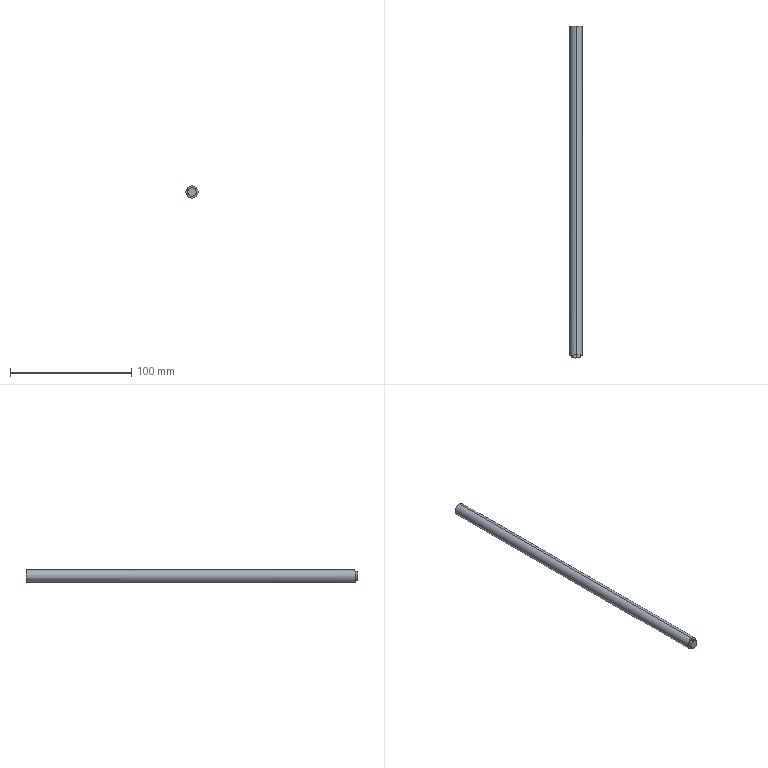Part | Creo | 1 solid | 8 faces | box 10 x 273.752 x 10 mm | volume 21397 mm3 | plane 4 | cylinder 4 | commonest cylinder face diameters 7.035 x2 10 x2
STEP:
#1=CARTESIAN_POINT('',(0.,0.,0.));
#2=DIRECTION('',(0.,0.,1.));
#3=DIRECTION('',(1.,0.,0.));
#4=AXIS2_PLACEMENT_3D('',#1,#2,#3);
#5=CARTESIAN_POINT('',(90.074,305.373,-76.269));
#6=VERTEX_POINT('',#5);
#7=CARTESIAN_POINT('',(85.074,305.373,-81.269));
#8=VERTEX_POINT('',#7);
#9=CARTESIAN_POINT('',(85.074,305.373,-76.269));
#10=DIRECTION('',(0.,1.,0.));
#11=DIRECTION('',(1.,0.,0.));
#12=AXIS2_PLACEMENT_3D('',#9,#10,#11);
#13=CIRCLE('',#12,5.);
#14=EDGE_CURVE('',#6,#8,#13,.T.);
#15=ORIENTED_EDGE('',*,*,#14,.F.);
#16=CARTESIAN_POINT('',(85.074,305.373,-71.269));
#17=VERTEX_POINT('',#16);
#18=CARTESIAN_POINT('',(85.074,305.373,-76.269));
#19=DIRECTION('',(0.,1.,0.));
#20=DIRECTION('',(0.,0.,1.));
#21=AXIS2_PLACEMENT_3D('',#18,#19,#20);
#22=CIRCLE('',#21,5.);
#23=EDGE_CURVE('',#17,#6,#22,.T.);
#24=ORIENTED_EDGE('',*,*,#23,.F.);
#25=CARTESIAN_POINT('',(85.074,305.373,-76.269));
#26=DIRECTION('',(0.,1.,0.));
#27=DIRECTION('',(0.,0.,-1.));
#28=AXIS2_PLACEMENT_3D('',#25,#26,#27);
#29=CIRCLE('',#28,5.);
#30=EDGE_CURVE('',#8,#17,#29,.T.);
#31=ORIENTED_EDGE('',*,*,#30,.F.);
#32=EDGE_LOOP('',(#15,#24,#31));
#33=FACE_OUTER_BOUND('',#32,.F.);
#34=CARTESIAN_POINT('',(-335.899,305.373,-228.441));
#35=DIRECTION('',(0.,-1.,0.));
#36=DIRECTION('',(1.,0.,0.));
#37=AXIS2_PLACEMENT_3D('',#34,#35,#36);
#38=PLANE('',#37);
#39=ADVANCED_FACE('',(#33),#38,.F.);
#40=CARTESIAN_POINT('',(85.074,34.139,-71.269));
#41=VERTEX_POINT('',#40);
#42=CARTESIAN_POINT('',(85.075,33.964,-81.269));
#43=VERTEX_POINT('',#42);
#44=CARTESIAN_POINT('',(85.074,34.139,-71.269));
#45=CARTESIAN_POINT('',(85.307,34.139,-71.269));
#46=CARTESIAN_POINT('',(85.767,34.139,-71.301));
#47=CARTESIAN_POINT('',(86.449,34.137,-71.445));
#48=CARTESIAN_POINT('',(87.103,34.133,-71.682));
#49=CARTESIAN_POINT('',(87.718,34.128,-72.007));
#50=CARTESIAN_POINT('',(88.283,34.121,-72.414));
#51=CARTESIAN_POINT('',(88.785,34.113,-72.895));
#52=CARTESIAN_POINT('',(89.217,34.104,-73.441));
#53=CARTESIAN_POINT('',(89.568,34.094,-74.042));
#54=CARTESIAN_POINT('',(89.833,34.083,-74.685));
#55=CARTESIAN_POINT('',(90.007,34.071,-75.359));
#56=CARTESIAN_POINT('',(90.085,34.059,-76.051));
#57=CARTESIAN_POINT('',(90.067,34.047,-76.746));
#58=CARTESIAN_POINT('',(89.953,34.035,-77.433));
#59=CARTESIAN_POINT('',(89.745,34.023,-78.097));
#60=CARTESIAN_POINT('',(89.447,34.012,-78.726));
#61=CARTESIAN_POINT('',(89.065,34.002,-79.307));
#62=CARTESIAN_POINT('',(88.606,33.992,-79.831));
#63=CARTESIAN_POINT('',(88.079,33.984,-80.285));
#64=CARTESIAN_POINT('',(87.494,33.977,-80.662));
#65=CARTESIAN_POINT('',(86.86,33.971,-80.956));
#66=CARTESIAN_POINT('',(86.218,33.967,-81.149));
#67=CARTESIAN_POINT('',(85.657,33.965,-81.246));
#68=CARTESIAN_POINT('',(85.266,33.964,-81.269));
#69=CARTESIAN_POINT('',(85.075,33.964,-81.269));
#70=B_SPLINE_CURVE_WITH_KNOTS('',3,(#44,#45,#46,#47,#48,#49,#50,#51,#52,#53,#54,#55,#56,#57,#58,#59,#60,#61,#62,#63,#64,#65,#66,#67,#68,#69),.UNSPECIFIED.,.F.,.F.,(4,1,1,1,1,1,1,1,1,1,1,1,1,1,1,1,1,1,1,1,1,1,1,4),(0.,0.04348,0.08696,0.1304,0.1739,0.2174,0.2609,0.3043,0.3478,0.3913,0.4348,0.4783,0.5217,0.5652,0.6087,0.6522,0.6957,0.7391,0.7826,0.8261,0.8696,0.913,0.9565,1.),.UNSPECIFIED.);
#71=EDGE_CURVE('',#41,#43,#70,.T.);
#72=ORIENTED_EDGE('',*,*,#71,.F.);
#73=CARTESIAN_POINT('',(85.074,34.139,-71.269));
#74=DIRECTION('',(0.,1.,0.000000528));
#75=VECTOR('',#74,271.234);
#76=LINE('',#73,#75);
#77=EDGE_CURVE('',#41,#17,#76,.T.);
#78=ORIENTED_EDGE('',*,*,#77,.T.);
#79=ORIENTED_EDGE('',*,*,#23,.T.);
#80=ORIENTED_EDGE('',*,*,#14,.T.);
#81=CARTESIAN_POINT('',(85.075,33.964,-81.269));
#82=DIRECTION('',(-0.000005033,1.,-0.00000083));
#83=VECTOR('',#82,271.408);
#84=LINE('',#81,#83);
#85=EDGE_CURVE('',#43,#8,#84,.T.);
#86=ORIENTED_EDGE('',*,*,#85,.F.);
#87=EDGE_LOOP('',(#72,#78,#79,#80,#86));
#88=FACE_OUTER_BOUND('',#87,.F.);
#89=CARTESIAN_POINT('',(85.074,34.051,-76.269));
#90=DIRECTION('',(0.,1.,0.));
#91=DIRECTION('',(0.,0.,1.));
#92=AXIS2_PLACEMENT_3D('',#89,#90,#91);
#93=CYLINDRICAL_SURFACE('',#92,5.);
#94=ADVANCED_FACE('',(#88),#93,.T.);
#95=ORIENTED_EDGE('',*,*,#71,.T.);
#96=CARTESIAN_POINT('',(84.837,33.964,-81.263));
#97=VERTEX_POINT('',#96);
#98=CARTESIAN_POINT('',(85.075,33.964,-81.269));
#99=CARTESIAN_POINT('',(84.995,33.964,-81.269));
#100=CARTESIAN_POINT('',(84.917,33.964,-81.267));
#101=CARTESIAN_POINT('',(84.837,33.964,-81.263));
#102=B_SPLINE_CURVE_WITH_KNOTS('',3,(#98,#99,#100,#101),.UNSPECIFIED.,.F.,.F.,(4,4),(0.,1.),.UNSPECIFIED.);
#103=EDGE_CURVE('',#43,#97,#102,.T.);
#104=ORIENTED_EDGE('',*,*,#103,.T.);
#105=CARTESIAN_POINT('',(81.074,33.996,-79.269));
#106=VERTEX_POINT('',#105);
#107=CARTESIAN_POINT('',(84.465,33.964,-81.246));
#108=CARTESIAN_POINT('',(83.745,33.965,-81.13));
#109=CARTESIAN_POINT('',(82.713,33.972,-80.723));
#110=CARTESIAN_POINT('',(81.797,33.982,-80.098));
#111=CARTESIAN_POINT('',(81.297,33.991,-79.567));
#112=CARTESIAN_POINT('',(81.074,33.996,-79.269));
#113=B_SPLINE_CURVE_WITH_KNOTS('',3,(#96,#107,#108,#109,#110,#111,#112),.UNSPECIFIED.,.F.,.F.,(4,1,1,1,4),(0.,0.25,0.5,0.75,1.),.UNSPECIFIED.);
#114=EDGE_CURVE('',#97,#106,#113,.T.);
#115=ORIENTED_EDGE('',*,*,#114,.T.);
#116=CARTESIAN_POINT('',(81.074,34.1,-73.269));
#117=VERTEX_POINT('',#116);
#118=CARTESIAN_POINT('',(81.074,34.1,-73.269));
#119=DIRECTION('',(-0.000000019,-0.01745,-0.9998));
#120=VECTOR('',#119,6.001);
#121=LINE('',#118,#120);
#122=EDGE_CURVE('',#117,#106,#121,.T.);
#123=ORIENTED_EDGE('',*,*,#122,.F.);
#124=CARTESIAN_POINT('',(81.074,34.1,-73.269));
#125=CARTESIAN_POINT('',(81.309,34.106,-72.955));
#126=CARTESIAN_POINT('',(81.839,34.116,-72.398));
#127=CARTESIAN_POINT('',(82.817,34.128,-71.756));
#128=CARTESIAN_POINT('',(83.918,34.136,-71.359));
#129=CARTESIAN_POINT('',(84.68,34.138,-71.269));
#130=CARTESIAN_POINT('',(85.074,34.139,-71.269));
#131=B_SPLINE_CURVE_WITH_KNOTS('',3,(#124,#125,#126,#127,#128,#129,#130),.UNSPECIFIED.,.F.,.F.,(4,1,1,1,4),(0.,0.25,0.5,0.75,1.),.UNSPECIFIED.);
#132=EDGE_CURVE('',#117,#41,#131,.T.);
#133=ORIENTED_EDGE('',*,*,#132,.T.);
#134=EDGE_LOOP('',(#95,#104,#115,#123,#133));
#135=FACE_OUTER_BOUND('',#134,.F.);
#136=CARTESIAN_POINT('',(85.074,34.113,-72.751));
#137=VERTEX_POINT('',#136);
#138=CARTESIAN_POINT('',(85.074,33.99,-79.786));
#139=VERTEX_POINT('',#138);
#140=CARTESIAN_POINT('',(85.074,34.113,-72.751));
#141=CARTESIAN_POINT('',(85.416,34.113,-72.751));
#142=CARTESIAN_POINT('',(86.072,34.112,-72.847));
#143=CARTESIAN_POINT('',(87.,34.105,-73.268));
#144=CARTESIAN_POINT('',(87.766,34.094,-73.933));
#145=CARTESIAN_POINT('',(88.314,34.08,-74.785));
#146=CARTESIAN_POINT('',(88.6,34.063,-75.752));
#147=CARTESIAN_POINT('',(88.604,34.046,-76.762));
#148=CARTESIAN_POINT('',(88.322,34.028,-77.738));
#149=CARTESIAN_POINT('',(87.775,34.013,-78.596));
#150=CARTESIAN_POINT('',(87.009,34.001,-79.264));
#151=CARTESIAN_POINT('',(86.083,33.993,-79.688));
#152=CARTESIAN_POINT('',(85.421,33.99,-79.786));
#153=CARTESIAN_POINT('',(85.074,33.99,-79.786));
#154=B_SPLINE_CURVE_WITH_KNOTS('',3,(#140,#141,#142,#143,#144,#145,#146,#147,#148,#149,#150,#151,#152,#153),.UNSPECIFIED.,.F.,.F.,(4,1,1,1,1,1,1,1,1,1,1,4),(0.,0.09091,0.1818,0.2727,0.3636,0.4545,0.5455,0.6364,0.7273,0.8182,0.9091,1.),.UNSPECIFIED.);
#155=EDGE_CURVE('',#137,#139,#154,.T.);
#156=ORIENTED_EDGE('',*,*,#155,.F.);
#157=CARTESIAN_POINT('',(84.907,33.99,-79.782));
#158=VERTEX_POINT('',#157);
#159=CARTESIAN_POINT('',(84.907,33.99,-79.782));
#160=CARTESIAN_POINT('',(84.53,33.99,-79.765));
#161=CARTESIAN_POINT('',(83.823,33.992,-79.615));
#162=CARTESIAN_POINT('',(82.858,34.001,-79.075));
#163=CARTESIAN_POINT('',(82.111,34.014,-78.268));
#164=CARTESIAN_POINT('',(81.642,34.031,-77.27));
#165=CARTESIAN_POINT('',(81.501,34.05,-76.172));
#166=CARTESIAN_POINT('',(81.699,34.069,-75.094));
#167=CARTESIAN_POINT('',(82.214,34.086,-74.125));
#168=CARTESIAN_POINT('',(83.003,34.101,-73.355));
#169=CARTESIAN_POINT('',(83.996,34.11,-72.863));
#170=CARTESIAN_POINT('',(84.702,34.112,-72.751));
#171=CARTESIAN_POINT('',(85.074,34.113,-72.751));
#172=B_SPLINE_CURVE_WITH_KNOTS('',3,(#159,#160,#161,#162,#163,#164,#165,#166,#167,#168,#169,#170,#171),.UNSPECIFIED.,.F.,.F.,(4,1,1,1,1,1,1,1,1,1,4),(0.,0.1,0.2,0.3,0.4,0.5,0.6,0.7,0.8,0.9,1.),.UNSPECIFIED.);
#173=EDGE_CURVE('',#158,#137,#172,.T.);
#174=ORIENTED_EDGE('',*,*,#173,.F.);
#175=CARTESIAN_POINT('',(85.074,33.99,-79.786));
#176=CARTESIAN_POINT('',(85.018,33.99,-79.786));
#177=CARTESIAN_POINT('',(84.962,33.99,-79.785));
#178=B_SPLINE_CURVE_WITH_KNOTS('',3,(#175,#176,#177,#157),.UNSPECIFIED.,.F.,.F.,(4,4),(0.,1.),.UNSPECIFIED.);
#179=EDGE_CURVE('',#139,#158,#178,.T.);
#180=ORIENTED_EDGE('',*,*,#179,.F.);
#181=EDGE_LOOP('',(#156,#174,#180));
#182=FACE_BOUND('',#181,.F.);
#183=CARTESIAN_POINT('',(82.032,34.202,-67.473));
#184=DIRECTION('',(-0.0008272,0.9998,-0.01745));
#185=DIRECTION('',(0.,0.01745,0.9998));
#186=AXIS2_PLACEMENT_3D('',#183,#184,#185);
#187=PLANE('',#186);
#188=ADVANCED_FACE('',(#135,#182),#187,.F.);
#189=CARTESIAN_POINT('',(81.074,33.996,-79.269));
#190=CARTESIAN_POINT('',(80.811,34.002,-78.918));
#191=CARTESIAN_POINT('',(80.393,34.014,-78.176));
#192=CARTESIAN_POINT('',(80.059,34.036,-76.917));
#193=CARTESIAN_POINT('',(80.059,34.059,-75.621));
#194=CARTESIAN_POINT('',(80.393,34.081,-74.362));
#195=CARTESIAN_POINT('',(80.811,34.094,-73.62));
#196=CARTESIAN_POINT('',(81.074,34.1,-73.269));
#197=B_SPLINE_CURVE_WITH_KNOTS('',3,(#189,#190,#191,#192,#193,#194,#195,#196),.UNSPECIFIED.,.F.,.F.,(4,1,1,1,1,4),(0.,0.2,0.4,0.6,0.8,1.),.UNSPECIFIED.);
#198=EDGE_CURVE('',#106,#117,#197,.T.);
#199=ORIENTED_EDGE('',*,*,#198,.F.);
#200=ORIENTED_EDGE('',*,*,#114,.F.);
#201=ORIENTED_EDGE('',*,*,#103,.F.);
#202=ORIENTED_EDGE('',*,*,#85,.T.);
#203=ORIENTED_EDGE('',*,*,#30,.T.);
#204=ORIENTED_EDGE('',*,*,#77,.F.);
#205=ORIENTED_EDGE('',*,*,#132,.F.);
#206=EDGE_LOOP('',(#199,#200,#201,#202,#203,#204,#205));
#207=FACE_OUTER_BOUND('',#206,.F.);
#208=CARTESIAN_POINT('',(85.074,34.051,-76.269));
#209=DIRECTION('',(0.,1.,0.));
#210=DIRECTION('',(0.,0.,1.));
#211=AXIS2_PLACEMENT_3D('',#208,#209,#210);
#212=CYLINDRICAL_SURFACE('',#211,5.);
#213=ADVANCED_FACE('',(#207),#212,.T.);
#214=ORIENTED_EDGE('',*,*,#198,.T.);
#215=ORIENTED_EDGE('',*,*,#122,.T.);
#216=EDGE_LOOP('',(#214,#215));
#217=FACE_OUTER_BOUND('',#216,.F.);
#218=CARTESIAN_POINT('',(81.083,33.981,-80.128));
#219=DIRECTION('',(-0.0008272,0.9998,-0.01745));
#220=DIRECTION('',(0.,0.01745,0.9998));
#221=AXIS2_PLACEMENT_3D('',#218,#219,#220);
#222=PLANE('',#221);
#223=ADVANCED_FACE('',(#217),#222,.F.);
#224=ORIENTED_EDGE('',*,*,#155,.T.);
#225=CARTESIAN_POINT('',(85.074,31.744,-79.786));
#226=VERTEX_POINT('',#225);
#227=CARTESIAN_POINT('',(85.074,33.99,-79.786));
#228=DIRECTION('',(0.,-1.,0.));
#229=VECTOR('',#228,2.246);
#230=LINE('',#227,#229);
#231=EDGE_CURVE('',#139,#226,#230,.T.);
#232=ORIENTED_EDGE('',*,*,#231,.T.);
#233=CARTESIAN_POINT('',(85.074,31.621,-72.751));
#234=VERTEX_POINT('',#233);
#235=CARTESIAN_POINT('',(85.074,31.744,-79.786));
#236=CARTESIAN_POINT('',(85.488,31.744,-79.786));
#237=CARTESIAN_POINT('',(86.384,31.742,-79.635));
#238=CARTESIAN_POINT('',(87.635,31.729,-78.833));
#239=CARTESIAN_POINT('',(88.441,31.707,-77.57));
#240=CARTESIAN_POINT('',(88.666,31.685,-76.269));
#241=CARTESIAN_POINT('',(88.441,31.662,-74.968));
#242=CARTESIAN_POINT('',(87.635,31.639,-73.705));
#243=CARTESIAN_POINT('',(86.384,31.624,-72.902));
#244=CARTESIAN_POINT('',(85.488,31.621,-72.751));
#245=CARTESIAN_POINT('',(85.074,31.621,-72.751));
#246=B_SPLINE_CURVE_WITH_KNOTS('',3,(#235,#236,#237,#238,#239,#240,#241,#242,#243,#244,#245),.UNSPECIFIED.,.F.,.F.,(4,1,1,1,1,1,1,1,4),(0.,0.125,0.25,0.375,0.5,0.625,0.75,0.875,1.),.UNSPECIFIED.);
#247=EDGE_CURVE('',#226,#234,#246,.T.);
#248=ORIENTED_EDGE('',*,*,#247,.T.);
#249=CARTESIAN_POINT('',(85.074,34.113,-72.751));
#250=DIRECTION('',(-0.0001393,-1.,0.00001287));
#251=VECTOR('',#250,2.492);
#252=LINE('',#249,#251);
#253=EDGE_CURVE('',#137,#234,#252,.T.);
#254=ORIENTED_EDGE('',*,*,#253,.F.);
#255=EDGE_LOOP('',(#224,#232,#248,#254));
#256=FACE_OUTER_BOUND('',#255,.F.);
#257=CARTESIAN_POINT('',(85.074,34.063,-76.269));
#258=DIRECTION('',(0.,-1.,0.));
#259=DIRECTION('',(0.,0.,-1.));
#260=AXIS2_PLACEMENT_3D('',#257,#258,#259);
#261=CYLINDRICAL_SURFACE('',#260,3.517);
#262=ADVANCED_FACE('',(#256),#261,.T.);
#263=ORIENTED_EDGE('',*,*,#179,.T.);
#264=ORIENTED_EDGE('',*,*,#173,.T.);
#265=ORIENTED_EDGE('',*,*,#253,.T.);
#266=CARTESIAN_POINT('',(84.938,31.621,-72.754));
#267=VERTEX_POINT('',#266);
#268=CARTESIAN_POINT('',(85.074,31.621,-72.751));
#269=CARTESIAN_POINT('',(85.028,31.621,-72.751));
#270=CARTESIAN_POINT('',(84.983,31.621,-72.752));
#271=B_SPLINE_CURVE_WITH_KNOTS('',3,(#268,#269,#270,#266),.UNSPECIFIED.,.F.,.F.,(4,4),(0.,1.),.UNSPECIFIED.);
#272=EDGE_CURVE('',#234,#267,#271,.T.);
#273=ORIENTED_EDGE('',*,*,#272,.T.);
#274=CARTESIAN_POINT('',(84.938,31.621,-72.754));
#275=CARTESIAN_POINT('',(84.878,31.621,-72.756));
#276=CARTESIAN_POINT('',(84.836,31.621,-72.759));
#277=CARTESIAN_POINT('',(84.752,31.621,-72.766));
#278=CARTESIAN_POINT('',(84.659,31.621,-72.775));
#279=CARTESIAN_POINT('',(84.558,31.621,-72.789));
#280=CARTESIAN_POINT('',(84.463,31.621,-72.804));
#281=CARTESIAN_POINT('',(84.355,31.622,-72.825));
#282=CARTESIAN_POINT('',(84.244,31.622,-72.85));
#283=CARTESIAN_POINT('',(84.131,31.622,-72.879));
#284=CARTESIAN_POINT('',(84.031,31.623,-72.909));
#285=CARTESIAN_POINT('',(83.912,31.623,-72.948));
#286=CARTESIAN_POINT('',(83.781,31.624,-72.996));
#287=CARTESIAN_POINT('',(83.644,31.625,-73.054));
#288=CARTESIAN_POINT('',(83.481,31.626,-73.13));
#289=CARTESIAN_POINT('',(83.306,31.628,-73.225));
#290=CARTESIAN_POINT('',(83.124,31.63,-73.339));
#291=CARTESIAN_POINT('',(82.965,31.632,-73.452));
#292=CARTESIAN_POINT('',(82.822,31.633,-73.564));
#293=CARTESIAN_POINT('',(82.651,31.636,-73.714));
#294=CARTESIAN_POINT('',(82.467,31.639,-73.901));
#295=CARTESIAN_POINT('',(82.281,31.643,-74.124));
#296=CARTESIAN_POINT('',(82.123,31.647,-74.347));
#297=CARTESIAN_POINT('',(81.99,31.65,-74.57));
#298=CARTESIAN_POINT('',(81.878,31.654,-74.792));
#299=CARTESIAN_POINT('',(81.754,31.659,-75.087));
#300=CARTESIAN_POINT('',(81.641,31.666,-75.456));
#301=CARTESIAN_POINT('',(81.566,31.673,-75.897));
#302=CARTESIAN_POINT('',(81.548,31.681,-76.337));
#303=CARTESIAN_POINT('',(81.583,31.689,-76.776));
#304=CARTESIAN_POINT('',(81.675,31.696,-77.214));
#305=CARTESIAN_POINT('',(81.802,31.703,-77.578));
#306=CARTESIAN_POINT('',(81.938,31.708,-77.868));
#307=CARTESIAN_POINT('',(82.058,31.712,-78.086));
#308=CARTESIAN_POINT('',(82.2,31.716,-78.303));
#309=CARTESIAN_POINT('',(82.366,31.72,-78.52));
#310=CARTESIAN_POINT('',(82.56,31.724,-78.736));
#311=CARTESIAN_POINT('',(82.752,31.727,-78.915));
#312=CARTESIAN_POINT('',(82.928,31.729,-79.058));
#313=CARTESIAN_POINT('',(83.075,31.731,-79.165));
#314=CARTESIAN_POINT('',(83.239,31.733,-79.272));
#315=CARTESIAN_POINT('',(83.424,31.735,-79.379));
#316=CARTESIAN_POINT('',(83.604,31.737,-79.467));
#317=CARTESIAN_POINT('',(83.77,31.738,-79.537));
#318=CARTESIAN_POINT('',(83.908,31.739,-79.589));
#319=CARTESIAN_POINT('',(84.041,31.74,-79.632));
#320=CARTESIAN_POINT('',(84.162,31.741,-79.667));
#321=CARTESIAN_POINT('',(84.262,31.741,-79.692));
#322=CARTESIAN_POINT('',(84.377,31.742,-79.717));
#323=CARTESIAN_POINT('',(84.489,31.742,-79.738));
#324=CARTESIAN_POINT('',(84.597,31.743,-79.754));
#325=CARTESIAN_POINT('',(84.692,31.743,-79.766));
#326=CARTESIAN_POINT('',(84.795,31.743,-79.776));
#327=CARTESIAN_POINT('',(84.888,31.743,-79.782));
#328=CARTESIAN_POINT('',(84.972,31.744,-79.785));
#329=CARTESIAN_POINT('',(85.014,31.744,-79.786));
#330=CARTESIAN_POINT('',(85.074,31.744,-79.786));
#331=B_SPLINE_CURVE_WITH_KNOTS('',3,(#274,#275,#276,#277,#278,#279,#280,#281,#282,#283,#284,#285,#286,#287,#288,#289,#290,#291,#292,#293,#294,#295,#296,#297,#298,#299,#300,#301,#302,#303,#304,#305,#306,#307,#308,#309,#310,#311,#312,#313,#314,#315,#316,#317,#318,#319,#320,#321,#322,#323,#324,#325,#326,#327,#328,#329,#330),.UNSPECIFIED.,.F.,.F.,(4,1,1,1,1,1,1,1,1,1,1,1,1,1,1,1,1,1,1,1,1,1,1,1,1,1,1,1,1,1,1,1,1,1,1,1,1,1,1,1,1,1,1,1,1,1,1,1,1,1,1,1,1,1,4),(0.,0.0004883,0.0009766,0.001953,0.003906,0.005859,0.007812,0.01172,0.01562,0.01953,0.02344,0.03125,0.03906,0.04688,0.0625,0.07812,0.09375,0.1094,0.125,0.1562,0.1875,0.2188,0.25,0.2812,0.3125,0.375,0.4375,0.5,0.5625,0.625,0.6875,0.7188,0.75,0.7812,0.8125,0.8438,0.875,0.8906,0.9062,0.9219,0.9375,0.9531,0.9609,0.9688,0.9766,0.9805,0.9844,0.9883,0.9922,0.9941,0.9961,0.998,0.999,0.9995,1.),.UNSPECIFIED.);
#332=EDGE_CURVE('',#267,#226,#331,.T.);
#333=ORIENTED_EDGE('',*,*,#332,.T.);
#334=ORIENTED_EDGE('',*,*,#231,.F.);
#335=EDGE_LOOP('',(#263,#264,#265,#273,#333,#334));
#336=FACE_OUTER_BOUND('',#335,.F.);
#337=CARTESIAN_POINT('',(85.074,34.063,-76.269));
#338=DIRECTION('',(0.,-1.,0.));
#339=DIRECTION('',(0.,0.,-1.));
#340=AXIS2_PLACEMENT_3D('',#337,#338,#339);
#341=CYLINDRICAL_SURFACE('',#340,3.517);
#342=ADVANCED_FACE('',(#336),#341,.T.);
#343=ORIENTED_EDGE('',*,*,#332,.F.);
#344=ORIENTED_EDGE('',*,*,#272,.F.);
#345=ORIENTED_EDGE('',*,*,#247,.F.);
#346=EDGE_LOOP('',(#343,#344,#345));
#347=FACE_OUTER_BOUND('',#346,.F.);
#348=CARTESIAN_POINT('',(73.32,31.944,-91.74));
#349=DIRECTION('',(0.000675,-0.9998,-0.01746));
#350=DIRECTION('',(0.,0.01746,-0.9998));
#351=AXIS2_PLACEMENT_3D('',#348,#349,#350);
#352=PLANE('',#351);
#353=ADVANCED_FACE('',(#347),#352,.T.);
#354=CLOSED_SHELL('',(#39,#94,#188,#213,#223,#262,#342,#353));
#355=MANIFOLD_SOLID_BREP('',#354);
#356=(LENGTH_UNIT()NAMED_UNIT(*)SI_UNIT(.MILLI.,.METRE.));
#357=UNCERTAINTY_MEASURE_WITH_UNIT(LENGTH_MEASURE(0.02741),#356,'','');
#358=(NAMED_UNIT(*)PLANE_ANGLE_UNIT()SI_UNIT($,.RADIAN.));
#359=PLANE_ANGLE_MEASURE_WITH_UNIT(PLANE_ANGLE_MEASURE(0.01745),#358);
#360=(CONVERSION_BASED_UNIT('DEGREE',#359)NAMED_UNIT(*)PLANE_ANGLE_UNIT());
#361=(NAMED_UNIT(*)SI_UNIT($,.STERADIAN.)SOLID_ANGLE_UNIT());
#362=(GEOMETRIC_REPRESENTATION_CONTEXT(3)GLOBAL_UNCERTAINTY_ASSIGNED_CONTEXT((#357))GLOBAL_UNIT_ASSIGNED_CONTEXT((#356,#360,#361))REPRESENTATION_CONTEXT('',''));
#363=ADVANCED_BREP_SHAPE_REPRESENTATION('',(#4,#355),#362);